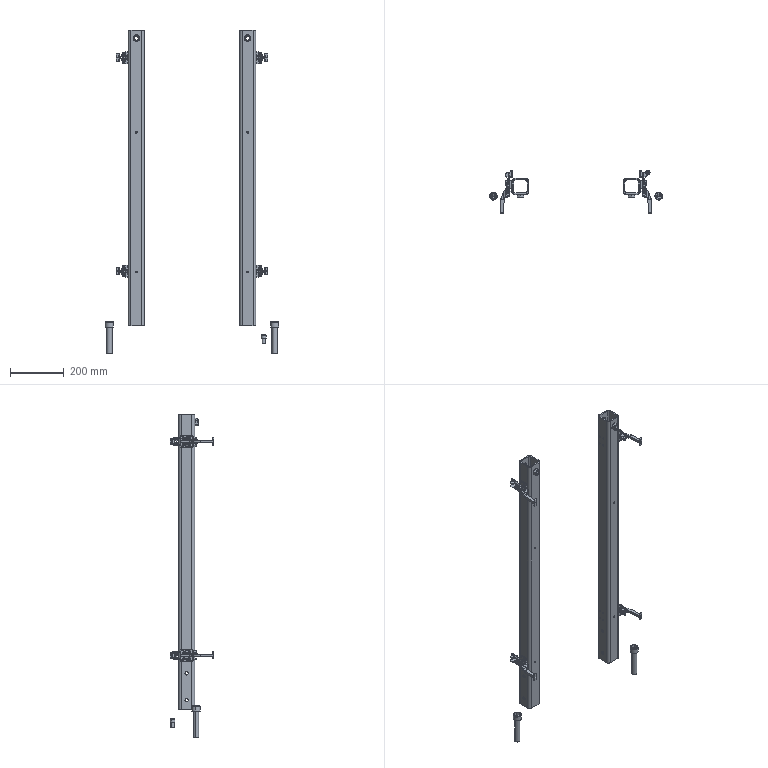Part | SolidWorks | features InContextFeatHolder 6 | 27 solids | 1191 faces | box 645 x 163.197 x 1205 mm | volume 2491880 mm3 | cylinder 560 | plane 537 | torus 46 | cone 40 | sphere 8 | commonest cylinder face diameters 6 x96 5 x72 3 x44 4 x32 6.7 x32 7 x32